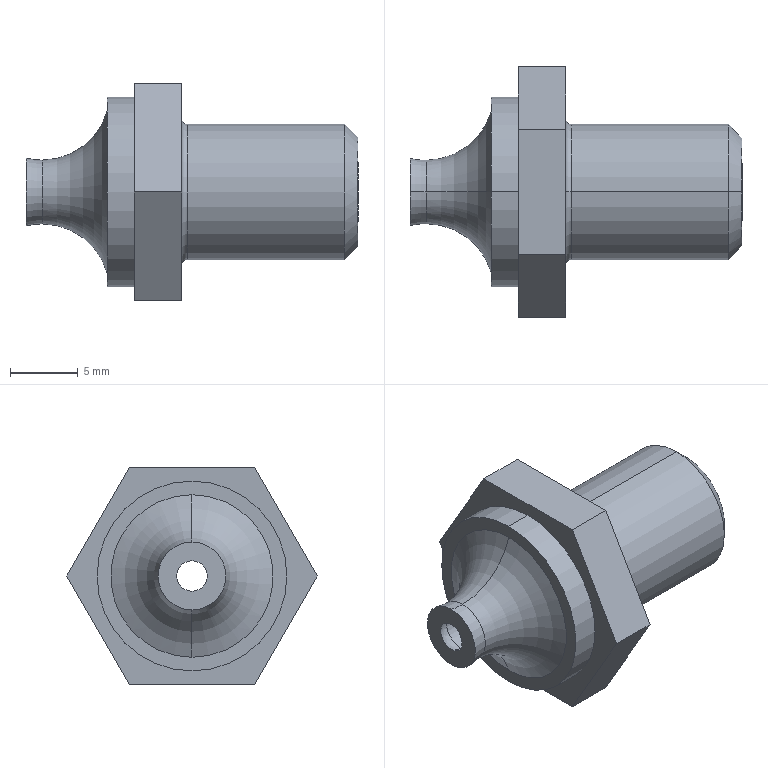Part | SolidWorks | features RevCut 6, Revolution 2, Chamfer 1, Cut 1, Extrusion 1, Fillet 1, LPattern 1 | 1 solid | 30 faces | box 24.5 x 18.475 x 16 mm | volume 2013 mm3 | plane 12 | cylinder 8 | torus 6 | sphere 2 | cone 2 | commonest cylinder face diameters 3 x2 4 x2 10 x2 14 x2
STEP:
#1=CARTESIAN_POINT('',(-5.1,0.,2.5));
#2=VERTEX_POINT('',#1);
#3=CARTESIAN_POINT('',(-3.912,0.,2.357));
#4=VERTEX_POINT('',#3);
#5=CARTESIAN_POINT('',(-3.912,0.,7.357));
#6=DIRECTION('',(0.,-1.,0.));
#7=DIRECTION('',(0.,0.,-1.));
#8=AXIS2_PLACEMENT_3D('',#5,#6,#7);
#9=CIRCLE('',#8,5.);
#10=EDGE_CURVE('',#2,#4,#9,.T.);
#11=ORIENTED_EDGE('',*,*,#10,.T.);
#12=CARTESIAN_POINT('',(-3.912,0.,-2.357));
#13=VERTEX_POINT('',#12);
#14=CARTESIAN_POINT('',(-3.912,0.,0.));
#15=DIRECTION('',(-1.,0.,0.));
#16=DIRECTION('',(0.,0.,1.));
#17=AXIS2_PLACEMENT_3D('',#14,#15,#16);
#18=CIRCLE('',#17,2.357);
#19=EDGE_CURVE('',#4,#13,#18,.T.);
#20=ORIENTED_EDGE('',*,*,#19,.T.);
#21=CARTESIAN_POINT('',(-5.1,0.,-2.5));
#22=VERTEX_POINT('',#21);
#23=CARTESIAN_POINT('',(-3.912,0.,-7.357));
#24=DIRECTION('',(0.,1.,0.));
#25=DIRECTION('',(0.,0.,1.));
#26=AXIS2_PLACEMENT_3D('',#23,#24,#25);
#27=CIRCLE('',#26,5.);
#28=EDGE_CURVE('',#22,#13,#27,.T.);
#29=ORIENTED_EDGE('',*,*,#28,.F.);
#30=CARTESIAN_POINT('',(-5.1,0.,0.));
#31=DIRECTION('',(-1.,0.,0.));
#32=DIRECTION('',(0.,0.,1.));
#33=AXIS2_PLACEMENT_3D('',#30,#31,#32);
#34=CIRCLE('',#33,2.5);
#35=EDGE_CURVE('',#2,#22,#34,.T.);
#36=ORIENTED_EDGE('',*,*,#35,.F.);
#37=EDGE_LOOP('',(#11,#20,#29,#36));
#38=FACE_OUTER_BOUND('',#37,.T.);
#39=CARTESIAN_POINT('',(-3.912,0.,0.));
#40=DIRECTION('',(-1.,0.,0.));
#41=DIRECTION('',(0.,0.,1.));
#42=AXIS2_PLACEMENT_3D('',#39,#40,#41);
#43=TOROIDAL_SURFACE('',#42,7.357,5.);
#44=ADVANCED_FACE('',(#38),#43,.F.);
#45=ORIENTED_EDGE('',*,*,#28,.T.);
#46=CARTESIAN_POINT('',(-3.912,0.,0.));
#47=DIRECTION('',(-1.,0.,0.));
#48=DIRECTION('',(0.,0.,1.));
#49=AXIS2_PLACEMENT_3D('',#46,#47,#48);
#50=CIRCLE('',#49,2.357);
#51=EDGE_CURVE('',#13,#4,#50,.T.);
#52=ORIENTED_EDGE('',*,*,#51,.T.);
#53=ORIENTED_EDGE('',*,*,#10,.F.);
#54=CARTESIAN_POINT('',(-5.1,0.,0.));
#55=DIRECTION('',(-1.,0.,0.));
#56=DIRECTION('',(0.,0.,1.));
#57=AXIS2_PLACEMENT_3D('',#54,#55,#56);
#58=CIRCLE('',#57,2.5);
#59=EDGE_CURVE('',#22,#2,#58,.T.);
#60=ORIENTED_EDGE('',*,*,#59,.F.);
#61=EDGE_LOOP('',(#45,#52,#53,#60));
#62=FACE_OUTER_BOUND('',#61,.T.);
#63=CARTESIAN_POINT('',(-3.912,0.,0.));
#64=DIRECTION('',(-1.,0.,0.));
#65=DIRECTION('',(0.,0.,1.));
#66=AXIS2_PLACEMENT_3D('',#63,#64,#65);
#67=TOROIDAL_SURFACE('',#66,7.357,5.);
#68=ADVANCED_FACE('',(#62),#67,.F.);
#69=CARTESIAN_POINT('',(19.4,0.,-2.));
#70=VERTEX_POINT('',#69);
#71=CARTESIAN_POINT('',(19.4,0.,2.));
#72=VERTEX_POINT('',#71);
#73=CARTESIAN_POINT('',(19.4,0.,0.));
#74=DIRECTION('',(-1.,0.,0.));
#75=DIRECTION('',(0.,0.,1.));
#76=AXIS2_PLACEMENT_3D('',#73,#74,#75);
#77=CIRCLE('',#76,2.);
#78=EDGE_CURVE('',#70,#72,#77,.T.);
#79=ORIENTED_EDGE('',*,*,#78,.F.);
#80=CARTESIAN_POINT('',(-0.2247,0.,-2.));
#81=VERTEX_POINT('',#80);
#82=CARTESIAN_POINT('',(-5.799,0.,-2.));
#83=DIRECTION('',(-1.,0.,0.));
#84=VECTOR('',#83,1000.);
#85=LINE('',#82,#84);
#86=EDGE_CURVE('',#70,#81,#85,.T.);
#87=ORIENTED_EDGE('',*,*,#86,.T.);
#88=CARTESIAN_POINT('',(-0.2247,0.,2.));
#89=VERTEX_POINT('',#88);
#90=CARTESIAN_POINT('',(-0.2247,0.,0.));
#91=DIRECTION('',(-1.,0.,0.));
#92=DIRECTION('',(0.,0.,1.));
#93=AXIS2_PLACEMENT_3D('',#90,#91,#92);
#94=CIRCLE('',#93,2.);
#95=EDGE_CURVE('',#81,#89,#94,.T.);
#96=ORIENTED_EDGE('',*,*,#95,.T.);
#97=CARTESIAN_POINT('',(-5.799,0.,2.));
#98=DIRECTION('',(-1.,0.,0.));
#99=VECTOR('',#98,1000.);
#100=LINE('',#97,#99);
#101=EDGE_CURVE('',#72,#89,#100,.T.);
#102=ORIENTED_EDGE('',*,*,#101,.F.);
#103=EDGE_LOOP('',(#79,#87,#96,#102));
#104=FACE_OUTER_BOUND('',#103,.T.);
#105=CARTESIAN_POINT('',(-5.799,0.,0.));
#106=DIRECTION('',(-1.,0.,0.));
#107=DIRECTION('',(0.,0.,1.));
#108=AXIS2_PLACEMENT_3D('',#105,#106,#107);
#109=CYLINDRICAL_SURFACE('',#108,2.);
#110=ADVANCED_FACE('',(#104),#109,.F.);
#111=CARTESIAN_POINT('',(-0.2247,0.,-1.5));
#112=VERTEX_POINT('',#111);
#113=CARTESIAN_POINT('',(-0.2247,0.,1.5));
#114=VERTEX_POINT('',#113);
#115=CARTESIAN_POINT('',(-0.2247,0.,0.));
#116=DIRECTION('',(-1.,0.,0.));
#117=DIRECTION('',(0.,0.,1.));
#118=AXIS2_PLACEMENT_3D('',#115,#116,#117);
#119=CIRCLE('',#118,1.5);
#120=EDGE_CURVE('',#112,#114,#119,.T.);
#121=ORIENTED_EDGE('',*,*,#120,.F.);
#122=CARTESIAN_POINT('',(-4.1,0.,-1.5));
#123=VERTEX_POINT('',#122);
#124=CARTESIAN_POINT('',(-5.799,0.,-1.5));
#125=DIRECTION('',(-1.,0.,0.));
#126=VECTOR('',#125,1000.);
#127=LINE('',#124,#126);
#128=EDGE_CURVE('',#112,#123,#127,.T.);
#129=ORIENTED_EDGE('',*,*,#128,.T.);
#130=CARTESIAN_POINT('',(-4.1,0.,1.5));
#131=VERTEX_POINT('',#130);
#132=CARTESIAN_POINT('',(-4.1,0.,0.));
#133=DIRECTION('',(-1.,0.,0.));
#134=DIRECTION('',(0.,0.,1.));
#135=AXIS2_PLACEMENT_3D('',#132,#133,#134);
#136=CIRCLE('',#135,1.5);
#137=EDGE_CURVE('',#123,#131,#136,.T.);
#138=ORIENTED_EDGE('',*,*,#137,.T.);
#139=CARTESIAN_POINT('',(-5.799,0.,1.5));
#140=DIRECTION('',(-1.,0.,0.));
#141=VECTOR('',#140,1000.);
#142=LINE('',#139,#141);
#143=EDGE_CURVE('',#114,#131,#142,.T.);
#144=ORIENTED_EDGE('',*,*,#143,.F.);
#145=EDGE_LOOP('',(#121,#129,#138,#144));
#146=FACE_OUTER_BOUND('',#145,.T.);
#147=CARTESIAN_POINT('',(-5.799,0.,0.));
#148=DIRECTION('',(-1.,0.,0.));
#149=DIRECTION('',(0.,0.,1.));
#150=AXIS2_PLACEMENT_3D('',#147,#148,#149);
#151=CYLINDRICAL_SURFACE('',#150,1.5);
#152=ADVANCED_FACE('',(#146),#151,.F.);
#153=CARTESIAN_POINT('',(-4.1,0.,0.));
#154=DIRECTION('',(-1.,0.,0.));
#155=DIRECTION('',(0.,0.,1.));
#156=AXIS2_PLACEMENT_3D('',#153,#154,#155);
#157=CIRCLE('',#156,1.5);
#158=EDGE_CURVE('',#131,#123,#157,.T.);
#159=ORIENTED_EDGE('',*,*,#158,.F.);
#160=CARTESIAN_POINT('',(-5.1,0.,1.118));
#161=VERTEX_POINT('',#160);
#162=CARTESIAN_POINT('',(-4.1,0.,0.));
#163=DIRECTION('',(0.,-1.,0.));
#164=DIRECTION('',(0.,0.,-1.));
#165=AXIS2_PLACEMENT_3D('',#162,#163,#164);
#166=CIRCLE('',#165,1.5);
#167=EDGE_CURVE('',#131,#161,#166,.T.);
#168=ORIENTED_EDGE('',*,*,#167,.T.);
#169=CARTESIAN_POINT('',(-5.1,0.,-1.118));
#170=VERTEX_POINT('',#169);
#171=CARTESIAN_POINT('',(-5.1,0.,0.));
#172=DIRECTION('',(-1.,0.,0.));
#173=DIRECTION('',(0.,0.,1.));
#174=AXIS2_PLACEMENT_3D('',#171,#172,#173);
#175=CIRCLE('',#174,1.118);
#176=EDGE_CURVE('',#161,#170,#175,.T.);
#177=ORIENTED_EDGE('',*,*,#176,.T.);
#178=CARTESIAN_POINT('',(-4.1,0.,0.));
#179=DIRECTION('',(0.,1.,0.));
#180=DIRECTION('',(0.,0.,1.));
#181=AXIS2_PLACEMENT_3D('',#178,#179,#180);
#182=CIRCLE('',#181,1.5);
#183=EDGE_CURVE('',#123,#170,#182,.T.);
#184=ORIENTED_EDGE('',*,*,#183,.F.);
#185=EDGE_LOOP('',(#159,#168,#177,#184));
#186=FACE_OUTER_BOUND('',#185,.T.);
#187=CARTESIAN_POINT('',(-4.1,0.,0.));
#188=DIRECTION('',(0.,-1.,0.));
#189=DIRECTION('',(0.,0.,-1.));
#190=AXIS2_PLACEMENT_3D('',#187,#188,#189);
#191=SPHERICAL_SURFACE('',#190,1.5);
#192=ADVANCED_FACE('',(#186),#191,.F.);
#193=CARTESIAN_POINT('',(2.9,0.,7.));
#194=VERTEX_POINT('',#193);
#195=CARTESIAN_POINT('',(2.9,0.,-7.));
#196=VERTEX_POINT('',#195);
#197=CARTESIAN_POINT('',(2.9,0.,0.));
#198=DIRECTION('',(-1.,0.,0.));
#199=DIRECTION('',(0.,0.,-1.));
#200=AXIS2_PLACEMENT_3D('',#197,#198,#199);
#201=CIRCLE('',#200,7.);
#202=EDGE_CURVE('',#194,#196,#201,.T.);
#203=ORIENTED_EDGE('',*,*,#202,.T.);
#204=CARTESIAN_POINT('',(0.9,0.,-7.));
#205=VERTEX_POINT('',#204);
#206=CARTESIAN_POINT('',(-7.318,0.,-7.));
#207=DIRECTION('',(-1.,0.,0.));
#208=VECTOR('',#207,1000.);
#209=LINE('',#206,#208);
#210=EDGE_CURVE('',#196,#205,#209,.T.);
#211=ORIENTED_EDGE('',*,*,#210,.T.);
#212=CARTESIAN_POINT('',(0.9,0.,7.));
#213=VERTEX_POINT('',#212);
#214=CARTESIAN_POINT('',(0.9,0.,0.));
#215=DIRECTION('',(-1.,0.,0.));
#216=DIRECTION('',(0.,0.,1.));
#217=AXIS2_PLACEMENT_3D('',#214,#215,#216);
#218=CIRCLE('',#217,7.);
#219=EDGE_CURVE('',#213,#205,#218,.T.);
#220=ORIENTED_EDGE('',*,*,#219,.F.);
#221=CARTESIAN_POINT('',(-7.318,0.,7.));
#222=DIRECTION('',(-1.,0.,0.));
#223=VECTOR('',#222,1000.);
#224=LINE('',#221,#223);
#225=EDGE_CURVE('',#194,#213,#224,.T.);
#226=ORIENTED_EDGE('',*,*,#225,.F.);
#227=EDGE_LOOP('',(#203,#211,#220,#226));
#228=FACE_OUTER_BOUND('',#227,.T.);
#229=CARTESIAN_POINT('',(-7.318,0.,0.));
#230=DIRECTION('',(-1.,0.,0.));
#231=DIRECTION('',(0.,0.,1.));
#232=AXIS2_PLACEMENT_3D('',#229,#230,#231);
#233=CYLINDRICAL_SURFACE('',#232,7.);
#234=ADVANCED_FACE('',(#228),#233,.T.);
#235=ORIENTED_EDGE('',*,*,#51,.F.);
#236=CARTESIAN_POINT('',(0.9,0.,-6.));
#237=VERTEX_POINT('',#236);
#238=CARTESIAN_POINT('',(-3.912,0.,-7.357));
#239=DIRECTION('',(0.,1.,0.));
#240=DIRECTION('',(0.,0.,1.));
#241=AXIS2_PLACEMENT_3D('',#238,#239,#240);
#242=CIRCLE('',#241,5.);
#243=EDGE_CURVE('',#13,#237,#242,.T.);
#244=ORIENTED_EDGE('',*,*,#243,.T.);
#245=CARTESIAN_POINT('',(0.9,0.,6.));
#246=VERTEX_POINT('',#245);
#247=CARTESIAN_POINT('',(0.9,0.,0.));
#248=DIRECTION('',(-1.,0.,0.));
#249=DIRECTION('',(0.,0.,1.));
#250=AXIS2_PLACEMENT_3D('',#247,#248,#249);
#251=CIRCLE('',#250,6.);
#252=EDGE_CURVE('',#237,#246,#251,.T.);
#253=ORIENTED_EDGE('',*,*,#252,.T.);
#254=CARTESIAN_POINT('',(-3.912,0.,7.357));
#255=DIRECTION('',(0.,-1.,0.));
#256=DIRECTION('',(0.,0.,-1.));
#257=AXIS2_PLACEMENT_3D('',#254,#255,#256);
#258=CIRCLE('',#257,5.);
#259=EDGE_CURVE('',#4,#246,#258,.T.);
#260=ORIENTED_EDGE('',*,*,#259,.F.);
#261=EDGE_LOOP('',(#235,#244,#253,#260));
#262=FACE_OUTER_BOUND('',#261,.T.);
#263=CARTESIAN_POINT('',(-3.912,0.,0.));
#264=DIRECTION('',(-1.,0.,0.));
#265=DIRECTION('',(0.,0.,1.));
#266=AXIS2_PLACEMENT_3D('',#263,#264,#265);
#267=TOROIDAL_SURFACE('',#266,7.357,5.);
#268=ADVANCED_FACE('',(#262),#267,.F.);
#269=CARTESIAN_POINT('',(19.4,0.,-4.));
#270=VERTEX_POINT('',#269);
#271=CARTESIAN_POINT('',(19.4,0.,4.));
#272=VERTEX_POINT('',#271);
#273=CARTESIAN_POINT('',(19.4,0.,0.));
#274=DIRECTION('',(1.,0.,0.));
#275=DIRECTION('',(0.,0.,-1.));
#276=AXIS2_PLACEMENT_3D('',#273,#274,#275);
#277=CIRCLE('',#276,4.);
#278=EDGE_CURVE('',#270,#272,#277,.T.);
#279=ORIENTED_EDGE('',*,*,#278,.F.);
#280=CARTESIAN_POINT('',(18.4,0.,-5.));
#281=VERTEX_POINT('',#280);
#282=CARTESIAN_POINT('',(18.4,0.,-5.));
#283=DIRECTION('',(-0.7071,0.,-0.7071));
#284=VECTOR('',#283,1000.);
#285=LINE('',#282,#284);
#286=EDGE_CURVE('',#270,#281,#285,.T.);
#287=ORIENTED_EDGE('',*,*,#286,.T.);
#288=CARTESIAN_POINT('',(18.4,0.,5.));
#289=VERTEX_POINT('',#288);
#290=CARTESIAN_POINT('',(18.4,0.,0.));
#291=DIRECTION('',(1.,0.,0.));
#292=DIRECTION('',(0.,0.,-1.));
#293=AXIS2_PLACEMENT_3D('',#290,#291,#292);
#294=CIRCLE('',#293,5.);
#295=EDGE_CURVE('',#281,#289,#294,.T.);
#296=ORIENTED_EDGE('',*,*,#295,.T.);
#297=CARTESIAN_POINT('',(18.4,0.,5.));
#298=DIRECTION('',(-0.7071,0.,0.7071));
#299=VECTOR('',#298,1000.);
#300=LINE('',#297,#299);
#301=EDGE_CURVE('',#272,#289,#300,.T.);
#302=ORIENTED_EDGE('',*,*,#301,.F.);
#303=EDGE_LOOP('',(#279,#287,#296,#302));
#304=FACE_OUTER_BOUND('',#303,.T.);
#305=CARTESIAN_POINT('',(18.4,0.,0.));
#306=DIRECTION('',(-1.,0.,0.));
#307=DIRECTION('',(0.,0.,1.));
#308=AXIS2_PLACEMENT_3D('',#305,#306,#307);
#309=CONICAL_SURFACE('',#308,5.,0.7854);
#310=ADVANCED_FACE('',(#304),#309,.T.);
#311=CARTESIAN_POINT('',(6.8,0.,5.));
#312=VERTEX_POINT('',#311);
#313=CARTESIAN_POINT('',(6.8,0.,-5.));
#314=VERTEX_POINT('',#313);
#315=CARTESIAN_POINT('',(6.8,0.,0.));
#316=DIRECTION('',(1.,0.,0.));
#317=DIRECTION('',(0.,0.,-1.));
#318=AXIS2_PLACEMENT_3D('',#315,#316,#317);
#319=CIRCLE('',#318,5.);
#320=EDGE_CURVE('',#312,#314,#319,.T.);
#321=ORIENTED_EDGE('',*,*,#320,.F.);
#322=CARTESIAN_POINT('',(6.4,0.,5.4));
#323=VERTEX_POINT('',#322);
#324=CARTESIAN_POINT('',(6.8,0.,5.4));
#325=DIRECTION('',(0.,1.,0.));
#326=DIRECTION('',(0.,0.,1.));
#327=AXIS2_PLACEMENT_3D('',#324,#325,#326);
#328=CIRCLE('',#327,0.4);
#329=EDGE_CURVE('',#312,#323,#328,.T.);
#330=ORIENTED_EDGE('',*,*,#329,.T.);
#331=CARTESIAN_POINT('',(6.4,0.,-5.4));
#332=VERTEX_POINT('',#331);
#333=CARTESIAN_POINT('',(6.4,0.,0.));
#334=DIRECTION('',(-1.,0.,0.));
#335=DIRECTION('',(0.,0.,-1.));
#336=AXIS2_PLACEMENT_3D('',#333,#334,#335);
#337=CIRCLE('',#336,5.4);
#338=EDGE_CURVE('',#332,#323,#337,.T.);
#339=ORIENTED_EDGE('',*,*,#338,.F.);
#340=CARTESIAN_POINT('',(6.8,0.,-5.4));
#341=DIRECTION('',(0.,-1.,0.));
#342=DIRECTION('',(0.,0.,-1.));
#343=AXIS2_PLACEMENT_3D('',#340,#341,#342);
#344=CIRCLE('',#343,0.4);
#345=EDGE_CURVE('',#314,#332,#344,.T.);
#346=ORIENTED_EDGE('',*,*,#345,.F.);
#347=EDGE_LOOP('',(#321,#330,#339,#346));
#348=FACE_OUTER_BOUND('',#347,.T.);
#349=CARTESIAN_POINT('',(6.8,0.,0.));
#350=DIRECTION('',(1.,0.,0.));
#351=DIRECTION('',(0.,0.,-1.));
#352=AXIS2_PLACEMENT_3D('',#349,#350,#351);
#353=TOROIDAL_SURFACE('',#352,5.4,0.4);
#354=ADVANCED_FACE('',(#348),#353,.F.);
#355=ORIENTED_EDGE('',*,*,#295,.F.);
#356=CARTESIAN_POINT('',(0.,0.,-5.));
#357=DIRECTION('',(-1.,0.,0.));
#358=VECTOR('',#357,1000.);
#359=LINE('',#356,#358);
#360=EDGE_CURVE('',#281,#314,#359,.T.);
#361=ORIENTED_EDGE('',*,*,#360,.T.);
#362=CARTESIAN_POINT('',(6.8,0.,0.));
#363=DIRECTION('',(1.,0.,0.));
#364=DIRECTION('',(0.,0.,-1.));
#365=AXIS2_PLACEMENT_3D('',#362,#363,#364);
#366=CIRCLE('',#365,5.);
#367=EDGE_CURVE('',#314,#312,#366,.T.);
#368=ORIENTED_EDGE('',*,*,#367,.T.);
#369=CARTESIAN_POINT('',(0.,0.,5.));
#370=DIRECTION('',(-1.,0.,0.));
#371=VECTOR('',#370,1000.);
#372=LINE('',#369,#371);
#373=EDGE_CURVE('',#289,#312,#372,.T.);
#374=ORIENTED_EDGE('',*,*,#373,.F.);
#375=EDGE_LOOP('',(#355,#361,#368,#374));
#376=FACE_OUTER_BOUND('',#375,.T.);
#377=CARTESIAN_POINT('',(0.,0.,0.));
#378=DIRECTION('',(-1.,0.,0.));
#379=DIRECTION('',(0.,0.,1.));
#380=AXIS2_PLACEMENT_3D('',#377,#378,#379);
#381=CYLINDRICAL_SURFACE('',#380,5.);
#382=ADVANCED_FACE('',(#376),#381,.T.);
#383=CARTESIAN_POINT('',(19.4,0.,0.));
#384=DIRECTION('',(1.,0.,0.));
#385=DIRECTION('',(0.,0.,-1.));
#386=AXIS2_PLACEMENT_3D('',#383,#384,#385);
#387=CIRCLE('',#386,4.);
#388=EDGE_CURVE('',#272,#270,#387,.T.);
#389=ORIENTED_EDGE('',*,*,#388,.T.);
#390=ORIENTED_EDGE('',*,*,#278,.T.);
#391=EDGE_LOOP('',(#389,#390));
#392=FACE_OUTER_BOUND('',#391,.T.);
#393=CARTESIAN_POINT('',(19.4,0.,0.));
#394=DIRECTION('',(-1.,0.,0.));
#395=DIRECTION('',(0.,0.,1.));
#396=AXIS2_PLACEMENT_3D('',#393,#394,#395);
#397=CIRCLE('',#396,2.);
#398=EDGE_CURVE('',#72,#70,#397,.T.);
#399=ORIENTED_EDGE('',*,*,#398,.T.);
#400=ORIENTED_EDGE('',*,*,#78,.T.);
#401=EDGE_LOOP('',(#399,#400));
#402=FACE_BOUND('',#401,.T.);
#403=CARTESIAN_POINT('',(19.4,0.,-4.));
#404=DIRECTION('',(-1.,0.,0.));
#405=DIRECTION('',(0.,0.,1.));
#406=AXIS2_PLACEMENT_3D('',#403,#404,#405);
#407=PLANE('',#406);
#408=ADVANCED_FACE('',(#392,#402),#407,.F.);
#409=ORIENTED_EDGE('',*,*,#35,.T.);
#410=ORIENTED_EDGE('',*,*,#59,.T.);
#411=EDGE_LOOP('',(#409,#410));
#412=FACE_OUTER_BOUND('',#411,.T.);
#413=CARTESIAN_POINT('',(-5.1,0.,0.));
#414=DIRECTION('',(-1.,0.,0.));
#415=DIRECTION('',(0.,0.,1.));
#416=AXIS2_PLACEMENT_3D('',#413,#414,#415);
#417=CIRCLE('',#416,1.118);
#418=EDGE_CURVE('',#170,#161,#417,.T.);
#419=ORIENTED_EDGE('',*,*,#418,.F.);
#420=ORIENTED_EDGE('',*,*,#176,.F.);
#421=EDGE_LOOP('',(#419,#420));
#422=FACE_BOUND('',#421,.T.);
#423=CARTESIAN_POINT('',(-5.1,0.,0.));
#424=DIRECTION('',(1.,0.,0.));
#425=DIRECTION('',(0.,0.,-1.));
#426=AXIS2_PLACEMENT_3D('',#423,#424,#425);
#427=PLANE('',#426);
#428=ADVANCED_FACE('',(#412,#422),#427,.F.);
#429=CARTESIAN_POINT('',(2.9,-4.619,-8.));
#430=VERTEX_POINT('',#429);
#431=CARTESIAN_POINT('',(2.9,4.619,-8.));
#432=VERTEX_POINT('',#431);
#433=CARTESIAN_POINT('',(2.9,-9.238,-8.));
#434=DIRECTION('',(0.,1.,0.));
#435=VECTOR('',#434,1000.);
#436=LINE('',#433,#435);
#437=EDGE_CURVE('',#430,#432,#436,.T.);
#438=ORIENTED_EDGE('',*,*,#437,.F.);
#439=CARTESIAN_POINT('',(2.9,-9.238,0.));
#440=VERTEX_POINT('',#439);
#441=CARTESIAN_POINT('',(2.9,-4.619,-8.));
#442=DIRECTION('',(0.,0.5,-0.866));
#443=VECTOR('',#442,1000.);
#444=LINE('',#441,#443);
#445=EDGE_CURVE('',#440,#430,#444,.T.);
#446=ORIENTED_EDGE('',*,*,#445,.F.);
#447=CARTESIAN_POINT('',(2.9,-4.619,8.));
#448=VERTEX_POINT('',#447);
#449=CARTESIAN_POINT('',(2.9,-9.238,0.));
#450=DIRECTION('',(0.,-0.5,-0.866));
#451=VECTOR('',#450,1000.);
#452=LINE('',#449,#451);
#453=EDGE_CURVE('',#448,#440,#452,.T.);
#454=ORIENTED_EDGE('',*,*,#453,.F.);
#455=CARTESIAN_POINT('',(2.9,4.619,8.));
#456=VERTEX_POINT('',#455);
#457=CARTESIAN_POINT('',(2.9,-9.238,8.));
#458=DIRECTION('',(0.,1.,0.));
#459=VECTOR('',#458,1000.);
#460=LINE('',#457,#459);
#461=EDGE_CURVE('',#448,#456,#460,.T.);
#462=ORIENTED_EDGE('',*,*,#461,.T.);
#463=CARTESIAN_POINT('',(2.9,9.238,0.));
#464=VERTEX_POINT('',#463);
#465=CARTESIAN_POINT('',(2.9,9.238,0.));
#466=DIRECTION('',(0.,-0.5,0.866));
#467=VECTOR('',#466,1000.);
#468=LINE('',#465,#467);
#469=EDGE_CURVE('',#464,#456,#468,.T.);
#470=ORIENTED_EDGE('',*,*,#469,.F.);
#471=CARTESIAN_POINT('',(2.9,4.619,-8.));
#472=DIRECTION('',(0.,0.5,0.866));
#473=VECTOR('',#472,1000.);
#474=LINE('',#471,#473);
#475=EDGE_CURVE('',#432,#464,#474,.T.);
#476=ORIENTED_EDGE('',*,*,#475,.F.);
#477=EDGE_LOOP('',(#438,#446,#454,#462,#470,#476));
#478=FACE_OUTER_BOUND('',#477,.T.);
#479=ORIENTED_EDGE('',*,*,#202,.F.);
#480=CARTESIAN_POINT('',(2.9,0.,0.));
#481=DIRECTION('',(-1.,0.,0.));
#482=DIRECTION('',(0.,0.,-1.));
#483=AXIS2_PLACEMENT_3D('',#480,#481,#482);
#484=CIRCLE('',#483,7.);
#485=EDGE_CURVE('',#196,#194,#484,.T.);
#486=ORIENTED_EDGE('',*,*,#485,.F.);
#487=EDGE_LOOP('',(#479,#486));
#488=FACE_BOUND('',#487,.T.);
#489=CARTESIAN_POINT('',(2.9,-9.238,-8.));
#490=DIRECTION('',(1.,0.,0.));
#491=DIRECTION('',(0.,0.,-1.));
#492=AXIS2_PLACEMENT_3D('',#489,#490,#491);
#493=PLANE('',#492);
#494=ADVANCED_FACE('',(#478,#488),#493,.F.);
#495=CARTESIAN_POINT('',(6.4,4.619,-8.));
#496=VERTEX_POINT('',#495);
#497=CARTESIAN_POINT('',(6.4,4.619,-8.));
#498=DIRECTION('',(-1.,0.,0.));
#499=VECTOR('',#498,1000.);
#500=LINE('',#497,#499);
#501=EDGE_CURVE('',#496,#432,#500,.T.);
#502=ORIENTED_EDGE('',*,*,#501,.T.);
#503=ORIENTED_EDGE('',*,*,#475,.T.);
#504=CARTESIAN_POINT('',(6.4,9.238,0.));
#505=VERTEX_POINT('',#504);
#506=CARTESIAN_POINT('',(6.4,9.238,0.));
#507=DIRECTION('',(-1.,0.,0.));
#508=VECTOR('',#507,1000.);
#509=LINE('',#506,#508);
#510=EDGE_CURVE('',#505,#464,#509,.T.);
#511=ORIENTED_EDGE('',*,*,#510,.F.);
#512=CARTESIAN_POINT('',(6.4,4.619,-8.));
#513=DIRECTION('',(0.,0.5,0.866));
#514=VECTOR('',#513,1000.);
#515=LINE('',#512,#514);
#516=EDGE_CURVE('',#496,#505,#515,.T.);
#517=ORIENTED_EDGE('',*,*,#516,.F.);
#518=EDGE_LOOP('',(#502,#503,#511,#517));
#519=FACE_OUTER_BOUND('',#518,.T.);
#520=CARTESIAN_POINT('',(6.4,4.619,-8.));
#521=DIRECTION('',(0.,-0.866,0.5));
#522=DIRECTION('',(0.,-0.5,-0.866));
#523=AXIS2_PLACEMENT_3D('',#520,#521,#522);
#524=PLANE('',#523);
#525=ADVANCED_FACE('',(#519),#524,.F.);
#526=ORIENTED_EDGE('',*,*,#510,.T.);
#527=ORIENTED_EDGE('',*,*,#469,.T.);
#528=CARTESIAN_POINT('',(6.4,4.619,8.));
#529=VERTEX_POINT('',#528);
#530=CARTESIAN_POINT('',(6.4,4.619,8.));
#531=DIRECTION('',(-1.,0.,0.));
#532=VECTOR('',#531,1000.);
#533=LINE('',#530,#532);
#534=EDGE_CURVE('',#529,#456,#533,.T.);
#535=ORIENTED_EDGE('',*,*,#534,.F.);
#536=CARTESIAN_POINT('',(6.4,9.238,0.));
#537=DIRECTION('',(0.,-0.5,0.866));
#538=VECTOR('',#537,1000.);
#539=LINE('',#536,#538);
#540=EDGE_CURVE('',#505,#529,#539,.T.);
#541=ORIENTED_EDGE('',*,*,#540,.F.);
#542=EDGE_LOOP('',(#526,#527,#535,#541));
#543=FACE_OUTER_BOUND('',#542,.T.);
#544=CARTESIAN_POINT('',(6.4,9.238,0.));
#545=DIRECTION('',(0.,-0.866,-0.5));
#546=DIRECTION('',(0.,0.5,-0.866));
#547=AXIS2_PLACEMENT_3D('',#544,#545,#546);
#548=PLANE('',#547);
#549=ADVANCED_FACE('',(#543),#548,.F.);
#550=ORIENTED_EDGE('',*,*,#534,.T.);
#551=ORIENTED_EDGE('',*,*,#461,.F.);
#552=CARTESIAN_POINT('',(6.4,-4.619,8.));
#553=VERTEX_POINT('',#552);
#554=CARTESIAN_POINT('',(6.4,-4.619,8.));
#555=DIRECTION('',(-1.,0.,0.));
#556=VECTOR('',#555,1000.);
#557=LINE('',#554,#556);
#558=EDGE_CURVE('',#553,#448,#557,.T.);
#559=ORIENTED_EDGE('',*,*,#558,.F.);
#560=CARTESIAN_POINT('',(6.4,4.619,8.));
#561=DIRECTION('',(0.,-1.,0.));
#562=VECTOR('',#561,1000.);
#563=LINE('',#560,#562);
#564=EDGE_CURVE('',#529,#553,#563,.T.);
#565=ORIENTED_EDGE('',*,*,#564,.F.);
#566=EDGE_LOOP('',(#550,#551,#559,#565));
#567=FACE_OUTER_BOUND('',#566,.T.);
#568=CARTESIAN_POINT('',(6.4,4.619,8.));
#569=DIRECTION('',(0.,0.,-1.));
#570=DIRECTION('',(0.,1.,0.));
#571=AXIS2_PLACEMENT_3D('',#568,#569,#570);
#572=PLANE('',#571);
#573=ADVANCED_FACE('',(#567),#572,.F.);
#574=ORIENTED_EDGE('',*,*,#558,.T.);
#575=ORIENTED_EDGE('',*,*,#453,.T.);
#576=CARTESIAN_POINT('',(6.4,-9.238,0.));
#577=VERTEX_POINT('',#576);
#578=CARTESIAN_POINT('',(6.4,-9.238,0.));
#579=DIRECTION('',(-1.,0.,0.));
#580=VECTOR('',#579,1000.);
#581=LINE('',#578,#580);
#582=EDGE_CURVE('',#577,#440,#581,.T.);
#583=ORIENTED_EDGE('',*,*,#582,.F.);
#584=CARTESIAN_POINT('',(6.4,-9.238,0.));
#585=DIRECTION('',(0.,-0.5,-0.866));
#586=VECTOR('',#585,1000.);
#587=LINE('',#584,#586);
#588=EDGE_CURVE('',#553,#577,#587,.T.);
#589=ORIENTED_EDGE('',*,*,#588,.F.);
#590=EDGE_LOOP('',(#574,#575,#583,#589));
#591=FACE_OUTER_BOUND('',#590,.T.);
#592=CARTESIAN_POINT('',(6.4,-9.238,0.));
#593=DIRECTION('',(0.,0.866,-0.5));
#594=DIRECTION('',(0.,0.5,0.866));
#595=AXIS2_PLACEMENT_3D('',#592,#593,#594);
#596=PLANE('',#595);
#597=ADVANCED_FACE('',(#591),#596,.F.);
#598=ORIENTED_EDGE('',*,*,#582,.T.);
#599=ORIENTED_EDGE('',*,*,#445,.T.);
#600=CARTESIAN_POINT('',(6.4,-4.619,-8.));
#601=VERTEX_POINT('',#600);
#602=CARTESIAN_POINT('',(6.4,-4.619,-8.));
#603=DIRECTION('',(-1.,0.,0.));
#604=VECTOR('',#603,1000.);
#605=LINE('',#602,#604);
#606=EDGE_CURVE('',#601,#430,#605,.T.);
#607=ORIENTED_EDGE('',*,*,#606,.F.);
#608=CARTESIAN_POINT('',(6.4,-4.619,-8.));
#609=DIRECTION('',(0.,0.5,-0.866));
#610=VECTOR('',#609,1000.);
#611=LINE('',#608,#610);
#612=EDGE_CURVE('',#577,#601,#611,.T.);
#613=ORIENTED_EDGE('',*,*,#612,.F.);
#614=EDGE_LOOP('',(#598,#599,#607,#613));
#615=FACE_OUTER_BOUND('',#614,.T.);
#616=CARTESIAN_POINT('',(6.4,-4.619,-8.));
#617=DIRECTION('',(0.,0.866,0.5));
#618=DIRECTION('',(0.,-0.5,0.866));
#619=AXIS2_PLACEMENT_3D('',#616,#617,#618);
#620=PLANE('',#619);
#621=ADVANCED_FACE('',(#615),#620,.F.);
#622=ORIENTED_EDGE('',*,*,#606,.T.);
#623=ORIENTED_EDGE('',*,*,#437,.T.);
#624=ORIENTED_EDGE('',*,*,#501,.F.);
#625=CARTESIAN_POINT('',(6.4,4.619,-8.));
#626=DIRECTION('',(0.,1.,0.));
#627=VECTOR('',#626,1000.);
#628=LINE('',#625,#627);
#629=EDGE_CURVE('',#601,#496,#628,.T.);
#630=ORIENTED_EDGE('',*,*,#629,.F.);
#631=EDGE_LOOP('',(#622,#623,#624,#630));
#632=FACE_OUTER_BOUND('',#631,.T.);
#633=CARTESIAN_POINT('',(6.4,4.619,-8.));
#634=DIRECTION('',(0.,0.,1.));
#635=DIRECTION('',(0.,-1.,0.));
#636=AXIS2_PLACEMENT_3D('',#633,#634,#635);
#637=PLANE('',#636);
#638=ADVANCED_FACE('',(#632),#637,.F.);
#639=ORIENTED_EDGE('',*,*,#338,.T.);
#640=CARTESIAN_POINT('',(6.4,0.,0.));
#641=DIRECTION('',(-1.,0.,0.));
#642=DIRECTION('',(0.,0.,-1.));
#643=AXIS2_PLACEMENT_3D('',#640,#641,#642);
#644=CIRCLE('',#643,5.4);
#645=EDGE_CURVE('',#323,#332,#644,.T.);
#646=ORIENTED_EDGE('',*,*,#645,.T.);
#647=EDGE_LOOP('',(#639,#646));
#648=FACE_BOUND('',#647,.T.);
#649=ORIENTED_EDGE('',*,*,#516,.T.);
#650=ORIENTED_EDGE('',*,*,#540,.T.);
#651=ORIENTED_EDGE('',*,*,#564,.T.);
#652=ORIENTED_EDGE('',*,*,#588,.T.);
#653=ORIENTED_EDGE('',*,*,#612,.T.);
#654=ORIENTED_EDGE('',*,*,#629,.T.);
#655=EDGE_LOOP('',(#649,#650,#651,#652,#653,#654));
#656=FACE_OUTER_BOUND('',#655,.T.);
#657=CARTESIAN_POINT('',(6.4,9.238,0.));
#658=DIRECTION('',(1.,0.,0.));
#659=DIRECTION('',(0.,0.,-1.));
#660=AXIS2_PLACEMENT_3D('',#657,#658,#659);
#661=PLANE('',#660);
#662=ADVANCED_FACE('',(#648,#656),#661,.T.);
#663=ORIENTED_EDGE('',*,*,#360,.F.);
#664=CARTESIAN_POINT('',(18.4,0.,0.));
#665=DIRECTION('',(1.,0.,0.));
#666=DIRECTION('',(0.,0.,-1.));
#667=AXIS2_PLACEMENT_3D('',#664,#665,#666);
#668=CIRCLE('',#667,5.);
#669=EDGE_CURVE('',#289,#281,#668,.T.);
#670=ORIENTED_EDGE('',*,*,#669,.F.);
#671=ORIENTED_EDGE('',*,*,#373,.T.);
#672=ORIENTED_EDGE('',*,*,#320,.T.);
#673=EDGE_LOOP('',(#663,#670,#671,#672));
#674=FACE_OUTER_BOUND('',#673,.T.);
#675=CARTESIAN_POINT('',(0.,0.,0.));
#676=DIRECTION('',(-1.,0.,0.));
#677=DIRECTION('',(0.,0.,1.));
#678=AXIS2_PLACEMENT_3D('',#675,#676,#677);
#679=CYLINDRICAL_SURFACE('',#678,5.);
#680=ADVANCED_FACE('',(#674),#679,.T.);
#681=ORIENTED_EDGE('',*,*,#329,.F.);
#682=ORIENTED_EDGE('',*,*,#367,.F.);
#683=ORIENTED_EDGE('',*,*,#345,.T.);
#684=ORIENTED_EDGE('',*,*,#645,.F.);
#685=EDGE_LOOP('',(#681,#682,#683,#684));
#686=FACE_OUTER_BOUND('',#685,.T.);
#687=CARTESIAN_POINT('',(6.8,0.,0.));
#688=DIRECTION('',(1.,0.,0.));
#689=DIRECTION('',(0.,0.,-1.));
#690=AXIS2_PLACEMENT_3D('',#687,#688,#689);
#691=TOROIDAL_SURFACE('',#690,5.4,0.4);
#692=ADVANCED_FACE('',(#686),#691,.F.);
#693=ORIENTED_EDGE('',*,*,#286,.F.);
#694=ORIENTED_EDGE('',*,*,#388,.F.);
#695=ORIENTED_EDGE('',*,*,#301,.T.);
#696=ORIENTED_EDGE('',*,*,#669,.T.);
#697=EDGE_LOOP('',(#693,#694,#695,#696));
#698=FACE_OUTER_BOUND('',#697,.T.);
#699=CARTESIAN_POINT('',(18.4,0.,0.));
#700=DIRECTION('',(-1.,0.,0.));
#701=DIRECTION('',(0.,0.,1.));
#702=AXIS2_PLACEMENT_3D('',#699,#700,#701);
#703=CONICAL_SURFACE('',#702,5.,0.7854);
#704=ADVANCED_FACE('',(#698),#703,.T.);
#705=ORIENTED_EDGE('',*,*,#19,.F.);
#706=ORIENTED_EDGE('',*,*,#259,.T.);
#707=CARTESIAN_POINT('',(0.9,0.,0.));
#708=DIRECTION('',(-1.,0.,0.));
#709=DIRECTION('',(0.,0.,1.));
#710=AXIS2_PLACEMENT_3D('',#707,#708,#709);
#711=CIRCLE('',#710,6.);
#712=EDGE_CURVE('',#246,#237,#711,.T.);
#713=ORIENTED_EDGE('',*,*,#712,.T.);
#714=ORIENTED_EDGE('',*,*,#243,.F.);
#715=EDGE_LOOP('',(#705,#706,#713,#714));
#716=FACE_OUTER_BOUND('',#715,.T.);
#717=CARTESIAN_POINT('',(-3.912,0.,0.));
#718=DIRECTION('',(-1.,0.,0.));
#719=DIRECTION('',(0.,0.,1.));
#720=AXIS2_PLACEMENT_3D('',#717,#718,#719);
#721=TOROIDAL_SURFACE('',#720,7.357,5.);
#722=ADVANCED_FACE('',(#716),#721,.F.);
#723=ORIENTED_EDGE('',*,*,#210,.F.);
#724=ORIENTED_EDGE('',*,*,#485,.T.);
#725=ORIENTED_EDGE('',*,*,#225,.T.);
#726=CARTESIAN_POINT('',(0.9,0.,0.));
#727=DIRECTION('',(-1.,0.,0.));
#728=DIRECTION('',(0.,0.,1.));
#729=AXIS2_PLACEMENT_3D('',#726,#727,#728);
#730=CIRCLE('',#729,7.);
#731=EDGE_CURVE('',#205,#213,#730,.T.);
#732=ORIENTED_EDGE('',*,*,#731,.F.);
#733=EDGE_LOOP('',(#723,#724,#725,#732));
#734=FACE_OUTER_BOUND('',#733,.T.);
#735=CARTESIAN_POINT('',(-7.318,0.,0.));
#736=DIRECTION('',(-1.,0.,0.));
#737=DIRECTION('',(0.,0.,1.));
#738=AXIS2_PLACEMENT_3D('',#735,#736,#737);
#739=CYLINDRICAL_SURFACE('',#738,7.);
#740=ADVANCED_FACE('',(#734),#739,.T.);
#741=ORIENTED_EDGE('',*,*,#712,.F.);
#742=ORIENTED_EDGE('',*,*,#252,.F.);
#743=EDGE_LOOP('',(#741,#742));
#744=FACE_BOUND('',#743,.T.);
#745=ORIENTED_EDGE('',*,*,#219,.T.);
#746=ORIENTED_EDGE('',*,*,#731,.T.);
#747=EDGE_LOOP('',(#745,#746));
#748=FACE_OUTER_BOUND('',#747,.T.);
#749=CARTESIAN_POINT('',(0.9,0.,-6.));
#750=DIRECTION('',(1.,0.,0.));
#751=DIRECTION('',(0.,0.,-1.));
#752=AXIS2_PLACEMENT_3D('',#749,#750,#751);
#753=PLANE('',#752);
#754=ADVANCED_FACE('',(#744,#748),#753,.F.);
#755=ORIENTED_EDGE('',*,*,#167,.F.);
#756=ORIENTED_EDGE('',*,*,#137,.F.);
#757=ORIENTED_EDGE('',*,*,#183,.T.);
#758=ORIENTED_EDGE('',*,*,#418,.T.);
#759=EDGE_LOOP('',(#755,#756,#757,#758));
#760=FACE_OUTER_BOUND('',#759,.T.);
#761=CARTESIAN_POINT('',(-4.1,0.,0.));
#762=DIRECTION('',(0.,-1.,0.));
#763=DIRECTION('',(0.,0.,-1.));
#764=AXIS2_PLACEMENT_3D('',#761,#762,#763);
#765=SPHERICAL_SURFACE('',#764,1.5);
#766=ADVANCED_FACE('',(#760),#765,.F.);
#767=ORIENTED_EDGE('',*,*,#128,.F.);
#768=CARTESIAN_POINT('',(-0.2247,0.,0.));
#769=DIRECTION('',(-1.,0.,0.));
#770=DIRECTION('',(0.,0.,1.));
#771=AXIS2_PLACEMENT_3D('',#768,#769,#770);
#772=CIRCLE('',#771,1.5);
#773=EDGE_CURVE('',#114,#112,#772,.T.);
#774=ORIENTED_EDGE('',*,*,#773,.F.);
#775=ORIENTED_EDGE('',*,*,#143,.T.);
#776=ORIENTED_EDGE('',*,*,#158,.T.);
#777=EDGE_LOOP('',(#767,#774,#775,#776));
#778=FACE_OUTER_BOUND('',#777,.T.);
#779=CARTESIAN_POINT('',(-5.799,0.,0.));
#780=DIRECTION('',(-1.,0.,0.));
#781=DIRECTION('',(0.,0.,1.));
#782=AXIS2_PLACEMENT_3D('',#779,#780,#781);
#783=CYLINDRICAL_SURFACE('',#782,1.5);
#784=ADVANCED_FACE('',(#778),#783,.F.);
#785=ORIENTED_EDGE('',*,*,#773,.T.);
#786=ORIENTED_EDGE('',*,*,#120,.T.);
#787=EDGE_LOOP('',(#785,#786));
#788=FACE_BOUND('',#787,.T.);
#789=CARTESIAN_POINT('',(-0.2247,0.,0.));
#790=DIRECTION('',(-1.,0.,0.));
#791=DIRECTION('',(0.,0.,1.));
#792=AXIS2_PLACEMENT_3D('',#789,#790,#791);
#793=CIRCLE('',#792,2.);
#794=EDGE_CURVE('',#89,#81,#793,.T.);
#795=ORIENTED_EDGE('',*,*,#794,.F.);
#796=ORIENTED_EDGE('',*,*,#95,.F.);
#797=EDGE_LOOP('',(#795,#796));
#798=FACE_OUTER_BOUND('',#797,.T.);
#799=CARTESIAN_POINT('',(-0.2247,0.,-2.));
#800=DIRECTION('',(1.,0.,0.));
#801=DIRECTION('',(0.,0.,-1.));
#802=AXIS2_PLACEMENT_3D('',#799,#800,#801);
#803=PLANE('',#802);
#804=ADVANCED_FACE('',(#788,#798),#803,.T.);
#805=ORIENTED_EDGE('',*,*,#86,.F.);
#806=ORIENTED_EDGE('',*,*,#398,.F.);
#807=ORIENTED_EDGE('',*,*,#101,.T.);
#808=ORIENTED_EDGE('',*,*,#794,.T.);
#809=EDGE_LOOP('',(#805,#806,#807,#808));
#810=FACE_OUTER_BOUND('',#809,.T.);
#811=CARTESIAN_POINT('',(-5.799,0.,0.));
#812=DIRECTION('',(-1.,0.,0.));
#813=DIRECTION('',(0.,0.,1.));
#814=AXIS2_PLACEMENT_3D('',#811,#812,#813);
#815=CYLINDRICAL_SURFACE('',#814,2.);
#816=ADVANCED_FACE('',(#810),#815,.F.);
#817=CLOSED_SHELL('',(#44,#68,#110,#152,#192,#234,#268,#310,#354,#382,#408,#428,#494,#525,#549,#573,#597,#621,#638,#662,#680,#692,#704,#722,#740,#754,#766,#784,#804,#816));
#818=MANIFOLD_SOLID_BREP('',#817);
#819=CARTESIAN_POINT('',(0.,0.,0.));
#820=DIRECTION('',(0.,0.,1.));
#821=DIRECTION('',(1.,0.,0.));
#822=AXIS2_PLACEMENT_3D('',#819,#820,#821);
#823=(LENGTH_UNIT()NAMED_UNIT(*)SI_UNIT(.MILLI.,.METRE.));
#824=UNCERTAINTY_MEASURE_WITH_UNIT(LENGTH_MEASURE(0.00001),#823,'','');
#825=(NAMED_UNIT(*)PLANE_ANGLE_UNIT()SI_UNIT($,.RADIAN.));
#826=(NAMED_UNIT(*)SI_UNIT($,.STERADIAN.)SOLID_ANGLE_UNIT());
#827=(GEOMETRIC_REPRESENTATION_CONTEXT(3)GLOBAL_UNCERTAINTY_ASSIGNED_CONTEXT((#824))GLOBAL_UNIT_ASSIGNED_CONTEXT((#823,#825,#826))REPRESENTATION_CONTEXT('',''));
#828=ADVANCED_BREP_SHAPE_REPRESENTATION('',(#818,#822),#827);